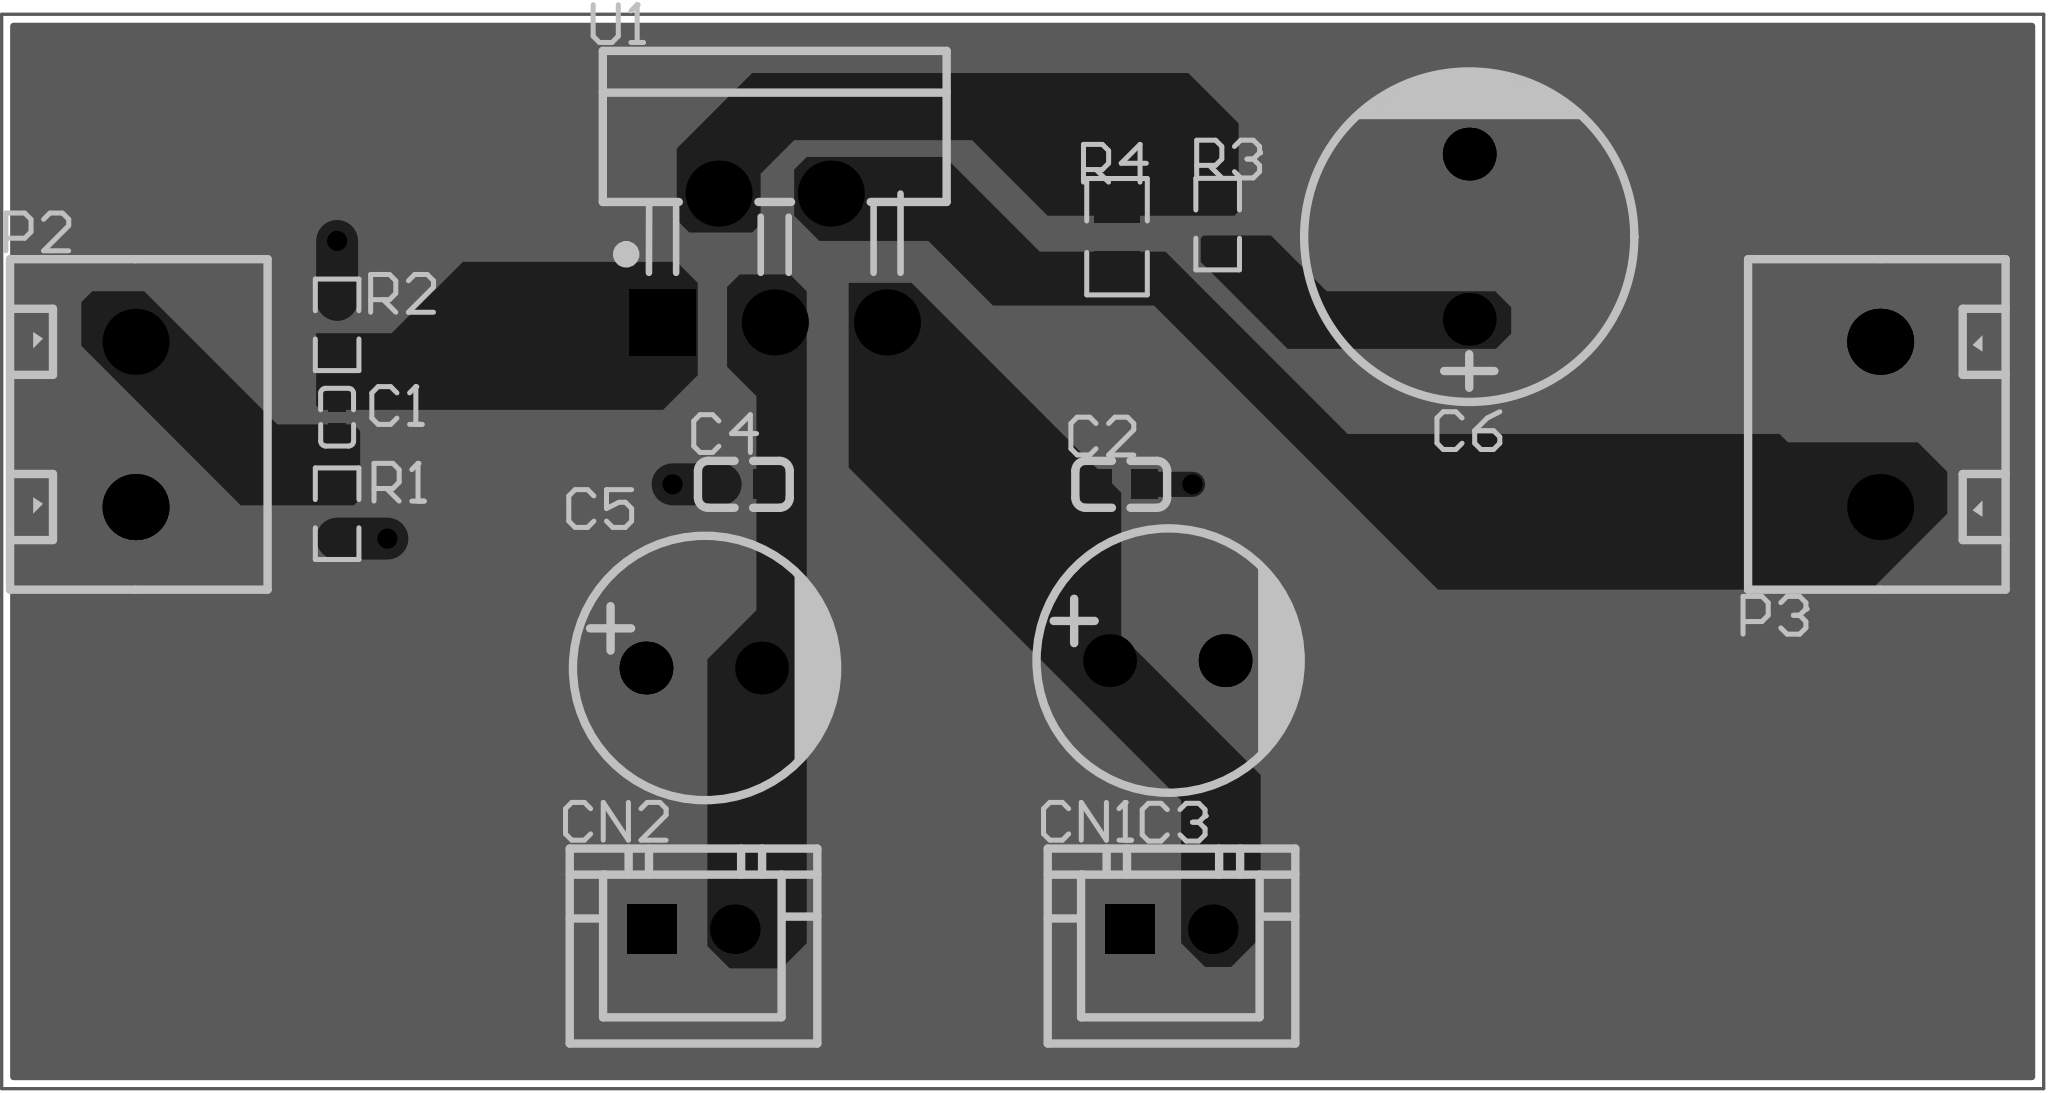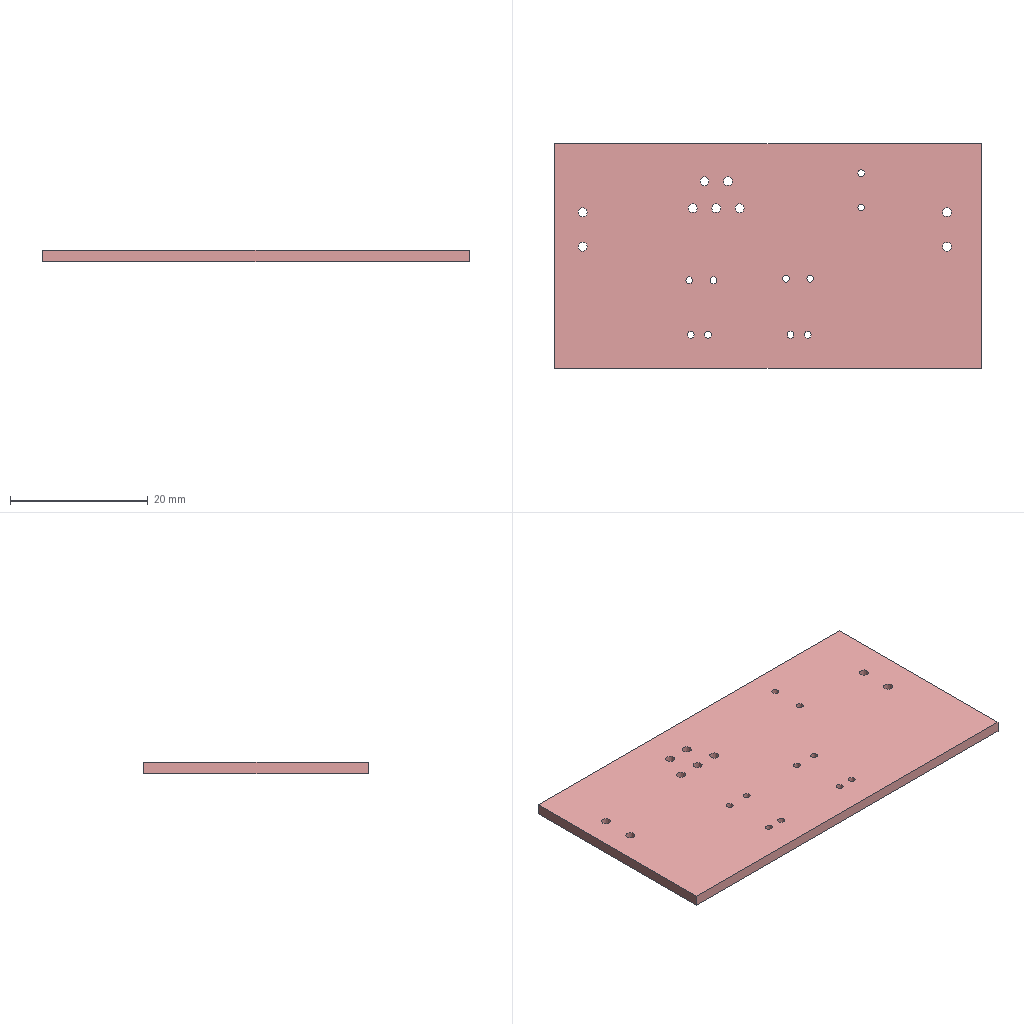Circuit board layout | Altium Designer | box 61.8 x 32.5 x 1.6 mm
Layer stack:
# Altium Designer layer stack of  (unit mm; dielectric type: 0 none, 1 core, 2 prepreg, 3 surface material)
index,name,kind,layer,copper_thickness_mm,dielectric_type,dielectric_thickness_mm,dielectric_material,dielectric_constant
0,Top Paste Mask Layer,other,,,,,,
1,Top Silkscreen Layer,other,,,,,,
2,Top Solder Mask Layer,dielectric,,,3,0.01,,3.3
3,Top Layer,copper,Top Layer,0.035,,,,
4,Dielectric1,dielectric,,,3,1.51,FR4,4.5
5,Bottom Layer,copper,Bottom Layer,0.035,,,,
6,Bottom Solder Mask Layer,dielectric,,,3,0.01,,3.3
7,Bottom Silkscreen Layer,other,,,,,,
8,Bottom Paste Mask Layer,other,,,,,,
# drill layer pairs: low layer,high layer
drill_pair,Top Layer,Bottom Layer
Part placement:
Designator,Comment,Layer,Footprint,Center-X(mm),Center-Y(mm),Rotation
C1,2.2uF,TopLayer,C0402,88.9,99.06,90
C2,100nF,TopLayer,C0603,112.649,97.028,180
C3,100uF,TopLayer,CAP-TH_BD8.0-P3.50-D0.5-FD,114.046,91.694,0
C4,100nF,TopLayer,C0603,101.219,97.028,0
C5,100uF,TopLayer,CAP-TH_BD8.0-P3.50-D0.5-FD,100.005,91.47,0
C6,22uF,TopLayer,CAP-TH_BD10.0-P5.00-D0.6-FD,123.19,104.521,90
CN1,HX-XH2.54-2PZZ,TopLayer,CONN-TH_2P-P2.50_HX-2.54MM-2P-ZZ-MS,114.173,83.566,0
CN2,HX-XH2.54-2PZZ,TopLayer,CONN-TH_2P-P2.50_HX-2.54MM-2P-ZZ-MS,99.695,83.566,0
P2,WJ126V-5.0-2P,TopLayer,CONN-TH_WJ126V-5.0-2P,82.794,98.84,0
P3,WJ126V-5.0-2P,TopLayer,CONN-TH_WJ126V-5.0-2P,135.636,98.841,180
R1,1MΩ,TopLayer,R0603,88.9,96.139,90
R2,22kΩ,TopLayer,R0603,88.9,101.854,270
R3,1kΩ,TopLayer,R0603,115.57,104.902,270
R4,100Ω,TopLayer,R0805,112.522,104.521,270
U1,TDA2030A,TopLayer,TO-220B-5_L10.6-W8.7-P1.70-BL,102.154,103.877,0
Pad and via stacks:
# Altium Designer via and pad stacks of  (unit mm). Each distinct definition once, with the count of objects using it.
# via: kind,start_layer,end_layer,hole_mm,diameter_mm,mode(0 simple;1 top-mid-bottom;2 full stack),diameter_per_layer,count,example_net
# pad: kind,layer,hole_mm,hole_type(0 round;1 square;2 slot),plating,top_size,top_shape(1 round;2 rect;3 octagon;9 rounded rect),mid_size,bottom_size,mode,footprint,size_per_layer,count,example
pad,Top Layer,0,0,plated,0.5x0.54,2,0.5x0.54,0.5x0.54,0,C0402,,2,C1.2
pad,Top Layer,0,0,plated,0.8x0.9,2,0.8x0.9,0.8x0.9,0,C0603,,4,C2.2
pad,Top Layer,0,0,plated,0.8065x0.864,2,0.8065x0.864,0.8065x0.864,0,R0603,,6,R1.2
pad,Top Layer,0,0,plated,1.133x1.377,2,1.133x1.377,1.133x1.377,0,R0805,,2,R4.2
pad,Multi-Layer,1,0,plated,1.6x1.6,1,1.6x1.6,1.6x1.6,0,CAP-TH_BD8.0-P3.50-D0.5-FD,,4,C3.1
pad,Multi-Layer,1,0,plated,1.6x1.6,1,1.6x1.6,1.6x1.6,0,CAP-TH_BD10.0-P5.00-D0.6-FD,,2,C6.2
pad,Multi-Layer,1,0,plated,1.5x1.5,2,1.5x1.5,1.5x1.5,0,CONN-TH_2P-P2.50_HX-2.54MM-2P-ZZ-MS,,2,CN1.1
pad,Multi-Layer,1,0,plated,1.5x1.5,1,1.5x1.5,1.5x1.5,0,CONN-TH_2P-P2.50_HX-2.54MM-2P-ZZ-MS,,2,CN1.2
pad,Multi-Layer,1.3,0,plated,2x2,1,2x2,2x2,0,CONN-TH_WJ126V-5.0-2P,,4,P2.1
pad,Multi-Layer,1.3,0,plated,2x2,1,2x2,2x2,0,TO-220B-5_L10.6-W8.7-P1.70-BL,,4,U1.5
pad,Multi-Layer,1.3,0,plated,2x2,2,2x2,2x2,0,TO-220B-5_L10.6-W8.7-P1.70-BL,,1,U1.1
via,Top Layer,Bottom Layer,0.3048,0.61,0,,4,GND
Copper pours:
name,layer,net,type(0 solid;1 hatched;2 none)
Bottom Layer-GND,Bottom Layer,GND,0
Design rules, without the lines most boards share:
# Altium Designer design rules of  (exported by Altium Designer, unit mm)
# columns: name | kind | enabled | priority | scope1 | scope2 | descriptor | typed fields (field=value)
creepage | 65 | enabled | 1 | All | All | Creepage Distance Constraint =(0mil) (All),(All) |